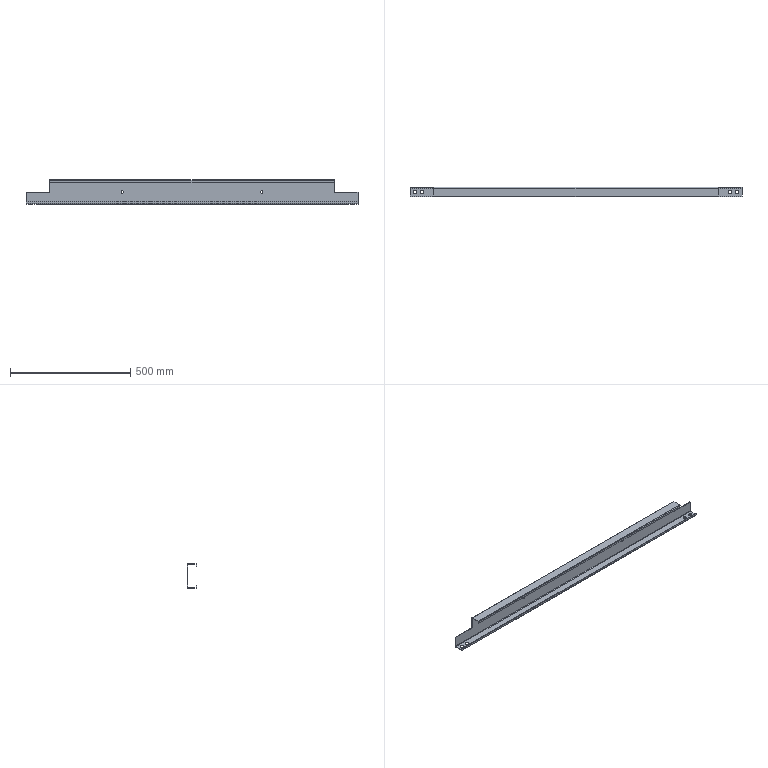Part | SolidWorks | features EdgeFlange 2, ICE 2, FlatPattern 1, SMBaseFlange 1, SheetMetal 1 | 1 solid | 54 faces | box 1380 x 40 x 100 mm | volume 478771 mm3 | plane 34 | cylinder 20 | commonest cylinder face diameters 15 x8 10 x4 2 x2 4 x2 6 x2 8 x2
STEP:
#1=CARTESIAN_POINT('',(-1204.379,-27.5,-98.));
#2=VERTEX_POINT('',#1);
#3=CARTESIAN_POINT('',(-1204.379,-12.5,-98.));
#4=VERTEX_POINT('',#3);
#5=CARTESIAN_POINT('',(-1204.379,-20.,-98.));
#6=DIRECTION('',(0.,0.,-1.));
#7=DIRECTION('',(0.,1.,0.));
#8=AXIS2_PLACEMENT_3D('',#5,#6,#7);
#9=CIRCLE('',#8,7.5);
#10=EDGE_CURVE('',#2,#4,#9,.T.);
#11=ORIENTED_EDGE('',*,*,#10,.F.);
#12=CARTESIAN_POINT('',(-1204.379,-27.5,-100.));
#13=VERTEX_POINT('',#12);
#14=CARTESIAN_POINT('',(-1204.379,-27.5,-90.));
#15=DIRECTION('',(0.,0.,-1.));
#16=VECTOR('',#15,1000.);
#17=LINE('',#14,#16);
#18=EDGE_CURVE('',#2,#13,#17,.T.);
#19=ORIENTED_EDGE('',*,*,#18,.T.);
#20=CARTESIAN_POINT('',(-1204.379,-12.5,-100.));
#21=VERTEX_POINT('',#20);
#22=CARTESIAN_POINT('',(-1204.379,-20.,-100.));
#23=DIRECTION('',(0.,0.,-1.));
#24=DIRECTION('',(0.,1.,0.));
#25=AXIS2_PLACEMENT_3D('',#22,#23,#24);
#26=CIRCLE('',#25,7.5);
#27=EDGE_CURVE('',#13,#21,#26,.T.);
#28=ORIENTED_EDGE('',*,*,#27,.T.);
#29=CARTESIAN_POINT('',(-1204.379,-12.5,-90.));
#30=DIRECTION('',(0.,0.,-1.));
#31=VECTOR('',#30,1000.);
#32=LINE('',#29,#31);
#33=EDGE_CURVE('',#4,#21,#32,.T.);
#34=ORIENTED_EDGE('',*,*,#33,.F.);
#35=EDGE_LOOP('',(#11,#19,#28,#34));
#36=FACE_OUTER_BOUND('',#35,.T.);
#37=CARTESIAN_POINT('',(-1204.379,-20.,-90.));
#38=DIRECTION('',(0.,0.,-1.));
#39=DIRECTION('',(0.,1.,0.));
#40=AXIS2_PLACEMENT_3D('',#37,#38,#39);
#41=CYLINDRICAL_SURFACE('',#40,7.5);
#42=ADVANCED_FACE('',(#36),#41,.F.);
#43=CARTESIAN_POINT('',(-1234.379,-27.5,-98.));
#44=VERTEX_POINT('',#43);
#45=CARTESIAN_POINT('',(-1234.379,-12.5,-98.));
#46=VERTEX_POINT('',#45);
#47=CARTESIAN_POINT('',(-1234.379,-20.,-98.));
#48=DIRECTION('',(0.,0.,-1.));
#49=DIRECTION('',(0.,1.,0.));
#50=AXIS2_PLACEMENT_3D('',#47,#48,#49);
#51=CIRCLE('',#50,7.5);
#52=EDGE_CURVE('',#44,#46,#51,.T.);
#53=ORIENTED_EDGE('',*,*,#52,.F.);
#54=CARTESIAN_POINT('',(-1234.379,-27.5,-100.));
#55=VERTEX_POINT('',#54);
#56=CARTESIAN_POINT('',(-1234.379,-27.5,-90.));
#57=DIRECTION('',(0.,0.,-1.));
#58=VECTOR('',#57,1000.);
#59=LINE('',#56,#58);
#60=EDGE_CURVE('',#44,#55,#59,.T.);
#61=ORIENTED_EDGE('',*,*,#60,.T.);
#62=CARTESIAN_POINT('',(-1234.379,-12.5,-100.));
#63=VERTEX_POINT('',#62);
#64=CARTESIAN_POINT('',(-1234.379,-20.,-100.));
#65=DIRECTION('',(0.,0.,-1.));
#66=DIRECTION('',(0.,1.,0.));
#67=AXIS2_PLACEMENT_3D('',#64,#65,#66);
#68=CIRCLE('',#67,7.5);
#69=EDGE_CURVE('',#55,#63,#68,.T.);
#70=ORIENTED_EDGE('',*,*,#69,.T.);
#71=CARTESIAN_POINT('',(-1234.379,-12.5,-90.));
#72=DIRECTION('',(0.,0.,-1.));
#73=VECTOR('',#72,1000.);
#74=LINE('',#71,#73);
#75=EDGE_CURVE('',#46,#63,#74,.T.);
#76=ORIENTED_EDGE('',*,*,#75,.F.);
#77=EDGE_LOOP('',(#53,#61,#70,#76));
#78=FACE_OUTER_BOUND('',#77,.T.);
#79=CARTESIAN_POINT('',(-1234.379,-20.,-90.));
#80=DIRECTION('',(0.,0.,-1.));
#81=DIRECTION('',(0.,1.,0.));
#82=AXIS2_PLACEMENT_3D('',#79,#80,#81);
#83=CYLINDRICAL_SURFACE('',#82,7.5);
#84=ADVANCED_FACE('',(#78),#83,.F.);
#85=CARTESIAN_POINT('',(75.621,-27.5,-98.));
#86=VERTEX_POINT('',#85);
#87=CARTESIAN_POINT('',(75.621,-12.5,-98.));
#88=VERTEX_POINT('',#87);
#89=CARTESIAN_POINT('',(75.621,-20.,-98.));
#90=DIRECTION('',(0.,0.,-1.));
#91=DIRECTION('',(0.,1.,0.));
#92=AXIS2_PLACEMENT_3D('',#89,#90,#91);
#93=CIRCLE('',#92,7.5);
#94=EDGE_CURVE('',#86,#88,#93,.T.);
#95=ORIENTED_EDGE('',*,*,#94,.F.);
#96=CARTESIAN_POINT('',(75.621,-27.5,-100.));
#97=VERTEX_POINT('',#96);
#98=CARTESIAN_POINT('',(75.621,-27.5,-90.));
#99=DIRECTION('',(0.,0.,-1.));
#100=VECTOR('',#99,1000.);
#101=LINE('',#98,#100);
#102=EDGE_CURVE('',#86,#97,#101,.T.);
#103=ORIENTED_EDGE('',*,*,#102,.T.);
#104=CARTESIAN_POINT('',(75.621,-12.5,-100.));
#105=VERTEX_POINT('',#104);
#106=CARTESIAN_POINT('',(75.621,-20.,-100.));
#107=DIRECTION('',(0.,0.,-1.));
#108=DIRECTION('',(0.,1.,0.));
#109=AXIS2_PLACEMENT_3D('',#106,#107,#108);
#110=CIRCLE('',#109,7.5);
#111=EDGE_CURVE('',#97,#105,#110,.T.);
#112=ORIENTED_EDGE('',*,*,#111,.T.);
#113=CARTESIAN_POINT('',(75.621,-12.5,-90.));
#114=DIRECTION('',(0.,0.,-1.));
#115=VECTOR('',#114,1000.);
#116=LINE('',#113,#115);
#117=EDGE_CURVE('',#88,#105,#116,.T.);
#118=ORIENTED_EDGE('',*,*,#117,.F.);
#119=EDGE_LOOP('',(#95,#103,#112,#118));
#120=FACE_OUTER_BOUND('',#119,.T.);
#121=CARTESIAN_POINT('',(75.621,-20.,-90.));
#122=DIRECTION('',(0.,0.,-1.));
#123=DIRECTION('',(0.,1.,0.));
#124=AXIS2_PLACEMENT_3D('',#121,#122,#123);
#125=CYLINDRICAL_SURFACE('',#124,7.5);
#126=ADVANCED_FACE('',(#120),#125,.F.);
#127=CARTESIAN_POINT('',(105.621,-27.5,-98.));
#128=VERTEX_POINT('',#127);
#129=CARTESIAN_POINT('',(105.621,-12.5,-98.));
#130=VERTEX_POINT('',#129);
#131=CARTESIAN_POINT('',(105.621,-20.,-98.));
#132=DIRECTION('',(0.,0.,-1.));
#133=DIRECTION('',(0.,1.,0.));
#134=AXIS2_PLACEMENT_3D('',#131,#132,#133);
#135=CIRCLE('',#134,7.5);
#136=EDGE_CURVE('',#128,#130,#135,.T.);
#137=ORIENTED_EDGE('',*,*,#136,.F.);
#138=CARTESIAN_POINT('',(105.621,-27.5,-100.));
#139=VERTEX_POINT('',#138);
#140=CARTESIAN_POINT('',(105.621,-27.5,-90.));
#141=DIRECTION('',(0.,0.,-1.));
#142=VECTOR('',#141,1000.);
#143=LINE('',#140,#142);
#144=EDGE_CURVE('',#128,#139,#143,.T.);
#145=ORIENTED_EDGE('',*,*,#144,.T.);
#146=CARTESIAN_POINT('',(105.621,-12.5,-100.));
#147=VERTEX_POINT('',#146);
#148=CARTESIAN_POINT('',(105.621,-20.,-100.));
#149=DIRECTION('',(0.,0.,-1.));
#150=DIRECTION('',(0.,1.,0.));
#151=AXIS2_PLACEMENT_3D('',#148,#149,#150);
#152=CIRCLE('',#151,7.5);
#153=EDGE_CURVE('',#139,#147,#152,.T.);
#154=ORIENTED_EDGE('',*,*,#153,.T.);
#155=CARTESIAN_POINT('',(105.621,-12.5,-90.));
#156=DIRECTION('',(0.,0.,-1.));
#157=VECTOR('',#156,1000.);
#158=LINE('',#155,#157);
#159=EDGE_CURVE('',#130,#147,#158,.T.);
#160=ORIENTED_EDGE('',*,*,#159,.F.);
#161=EDGE_LOOP('',(#137,#145,#154,#160));
#162=FACE_OUTER_BOUND('',#161,.T.);
#163=CARTESIAN_POINT('',(105.621,-20.,-90.));
#164=DIRECTION('',(0.,0.,-1.));
#165=DIRECTION('',(0.,1.,0.));
#166=AXIS2_PLACEMENT_3D('',#163,#164,#165);
#167=CYLINDRICAL_SURFACE('',#166,7.5);
#168=ADVANCED_FACE('',(#162),#167,.F.);
#169=CARTESIAN_POINT('',(-854.379,-2.,-55.));
#170=VERTEX_POINT('',#169);
#171=CARTESIAN_POINT('',(-854.379,-2.,-45.));
#172=VERTEX_POINT('',#171);
#173=CARTESIAN_POINT('',(-854.379,-2.,-50.));
#174=DIRECTION('',(0.,1.,0.));
#175=DIRECTION('',(0.,0.,1.));
#176=AXIS2_PLACEMENT_3D('',#173,#174,#175);
#177=CIRCLE('',#176,5.);
#178=EDGE_CURVE('',#170,#172,#177,.T.);
#179=ORIENTED_EDGE('',*,*,#178,.F.);
#180=CARTESIAN_POINT('',(-854.379,0.,-55.));
#181=VERTEX_POINT('',#180);
#182=CARTESIAN_POINT('',(-854.379,-2.,-55.));
#183=DIRECTION('',(0.,1.,0.));
#184=VECTOR('',#183,1000.);
#185=LINE('',#182,#184);
#186=EDGE_CURVE('',#170,#181,#185,.T.);
#187=ORIENTED_EDGE('',*,*,#186,.T.);
#188=CARTESIAN_POINT('',(-854.379,0.,-45.));
#189=VERTEX_POINT('',#188);
#190=CARTESIAN_POINT('',(-854.379,0.,-50.));
#191=DIRECTION('',(0.,1.,0.));
#192=DIRECTION('',(0.,0.,1.));
#193=AXIS2_PLACEMENT_3D('',#190,#191,#192);
#194=CIRCLE('',#193,5.);
#195=EDGE_CURVE('',#181,#189,#194,.T.);
#196=ORIENTED_EDGE('',*,*,#195,.T.);
#197=CARTESIAN_POINT('',(-854.379,-2.,-45.));
#198=DIRECTION('',(0.,1.,0.));
#199=VECTOR('',#198,1000.);
#200=LINE('',#197,#199);
#201=EDGE_CURVE('',#172,#189,#200,.T.);
#202=ORIENTED_EDGE('',*,*,#201,.F.);
#203=EDGE_LOOP('',(#179,#187,#196,#202));
#204=FACE_OUTER_BOUND('',#203,.T.);
#205=CARTESIAN_POINT('',(-854.379,-2.,-50.));
#206=DIRECTION('',(0.,1.,0.));
#207=DIRECTION('',(0.,0.,1.));
#208=AXIS2_PLACEMENT_3D('',#205,#206,#207);
#209=CYLINDRICAL_SURFACE('',#208,5.);
#210=ADVANCED_FACE('',(#204),#209,.F.);
#211=CARTESIAN_POINT('',(-274.379,-2.,-55.));
#212=VERTEX_POINT('',#211);
#213=CARTESIAN_POINT('',(-274.379,-2.,-45.));
#214=VERTEX_POINT('',#213);
#215=CARTESIAN_POINT('',(-274.379,-2.,-50.));
#216=DIRECTION('',(0.,1.,0.));
#217=DIRECTION('',(0.,0.,1.));
#218=AXIS2_PLACEMENT_3D('',#215,#216,#217);
#219=CIRCLE('',#218,5.);
#220=EDGE_CURVE('',#212,#214,#219,.T.);
#221=ORIENTED_EDGE('',*,*,#220,.F.);
#222=CARTESIAN_POINT('',(-274.379,0.,-55.));
#223=VERTEX_POINT('',#222);
#224=CARTESIAN_POINT('',(-274.379,-2.,-55.));
#225=DIRECTION('',(0.,1.,0.));
#226=VECTOR('',#225,1000.);
#227=LINE('',#224,#226);
#228=EDGE_CURVE('',#212,#223,#227,.T.);
#229=ORIENTED_EDGE('',*,*,#228,.T.);
#230=CARTESIAN_POINT('',(-274.379,0.,-45.));
#231=VERTEX_POINT('',#230);
#232=CARTESIAN_POINT('',(-274.379,0.,-50.));
#233=DIRECTION('',(0.,1.,0.));
#234=DIRECTION('',(0.,0.,1.));
#235=AXIS2_PLACEMENT_3D('',#232,#233,#234);
#236=CIRCLE('',#235,5.);
#237=EDGE_CURVE('',#223,#231,#236,.T.);
#238=ORIENTED_EDGE('',*,*,#237,.T.);
#239=CARTESIAN_POINT('',(-274.379,-2.,-45.));
#240=DIRECTION('',(0.,1.,0.));
#241=VECTOR('',#240,1000.);
#242=LINE('',#239,#241);
#243=EDGE_CURVE('',#214,#231,#242,.T.);
#244=ORIENTED_EDGE('',*,*,#243,.F.);
#245=EDGE_LOOP('',(#221,#229,#238,#244));
#246=FACE_OUTER_BOUND('',#245,.T.);
#247=CARTESIAN_POINT('',(-274.379,-2.,-50.));
#248=DIRECTION('',(0.,1.,0.));
#249=DIRECTION('',(0.,0.,1.));
#250=AXIS2_PLACEMENT_3D('',#247,#248,#249);
#251=CYLINDRICAL_SURFACE('',#250,5.);
#252=ADVANCED_FACE('',(#246),#251,.F.);
#253=CARTESIAN_POINT('',(-1156.379,-40.,-3.));
#254=VERTEX_POINT('',#253);
#255=CARTESIAN_POINT('',(-1156.379,-40.,-10.));
#256=VERTEX_POINT('',#255);
#257=CARTESIAN_POINT('',(-1156.379,-40.,0.));
#258=DIRECTION('',(0.,0.,-1.));
#259=VECTOR('',#258,1000.);
#260=LINE('',#257,#259);
#261=EDGE_CURVE('',#254,#256,#260,.T.);
#262=ORIENTED_EDGE('',*,*,#261,.F.);
#263=CARTESIAN_POINT('',(-1156.379,-38.,-3.));
#264=VERTEX_POINT('',#263);
#265=CARTESIAN_POINT('',(-1156.379,-40.,-3.));
#266=DIRECTION('',(0.,1.,0.));
#267=VECTOR('',#266,1000.);
#268=LINE('',#265,#267);
#269=EDGE_CURVE('',#254,#264,#268,.T.);
#270=ORIENTED_EDGE('',*,*,#269,.T.);
#271=CARTESIAN_POINT('',(-1156.379,-38.,-10.));
#272=VERTEX_POINT('',#271);
#273=CARTESIAN_POINT('',(-1156.379,-38.,0.));
#274=DIRECTION('',(0.,0.,-1.));
#275=VECTOR('',#274,1000.);
#276=LINE('',#273,#275);
#277=EDGE_CURVE('',#264,#272,#276,.T.);
#278=ORIENTED_EDGE('',*,*,#277,.T.);
#279=CARTESIAN_POINT('',(-1156.379,-40.,-10.));
#280=DIRECTION('',(0.,1.,0.));
#281=VECTOR('',#280,1000.);
#282=LINE('',#279,#281);
#283=EDGE_CURVE('',#256,#272,#282,.T.);
#284=ORIENTED_EDGE('',*,*,#283,.F.);
#285=EDGE_LOOP('',(#262,#270,#278,#284));
#286=FACE_OUTER_BOUND('',#285,.T.);
#287=CARTESIAN_POINT('',(-1156.379,24.338,-52.));
#288=DIRECTION('',(1.,0.,0.));
#289=DIRECTION('',(0.,0.,-1.));
#290=AXIS2_PLACEMENT_3D('',#287,#288,#289);
#291=PLANE('',#290);
#292=ADVANCED_FACE('',(#286),#291,.F.);
#293=CARTESIAN_POINT('',(-1156.379,-37.,-2.));
#294=VERTEX_POINT('',#293);
#295=CARTESIAN_POINT('',(-1156.379,-4.,-2.));
#296=VERTEX_POINT('',#295);
#297=CARTESIAN_POINT('',(-1156.379,0.,-2.));
#298=DIRECTION('',(0.,1.,0.));
#299=VECTOR('',#298,1000.);
#300=LINE('',#297,#299);
#301=EDGE_CURVE('',#294,#296,#300,.T.);
#302=ORIENTED_EDGE('',*,*,#301,.F.);
#303=CARTESIAN_POINT('',(-1156.379,-37.,0.));
#304=VERTEX_POINT('',#303);
#305=CARTESIAN_POINT('',(-1156.379,-37.,-2.));
#306=DIRECTION('',(0.,0.,1.));
#307=VECTOR('',#306,1000.);
#308=LINE('',#305,#307);
#309=EDGE_CURVE('',#294,#304,#308,.T.);
#310=ORIENTED_EDGE('',*,*,#309,.T.);
#311=CARTESIAN_POINT('',(-1156.379,-4.,0.));
#312=VERTEX_POINT('',#311);
#313=CARTESIAN_POINT('',(-1156.379,24.338,0.));
#314=DIRECTION('',(0.,1.,0.));
#315=VECTOR('',#314,1000.);
#316=LINE('',#313,#315);
#317=EDGE_CURVE('',#304,#312,#316,.T.);
#318=ORIENTED_EDGE('',*,*,#317,.T.);
#319=CARTESIAN_POINT('',(-1156.379,-4.,0.));
#320=DIRECTION('',(0.,0.,-1.));
#321=VECTOR('',#320,1000.);
#322=LINE('',#319,#321);
#323=EDGE_CURVE('',#312,#296,#322,.T.);
#324=ORIENTED_EDGE('',*,*,#323,.T.);
#325=EDGE_LOOP('',(#302,#310,#318,#324));
#326=FACE_OUTER_BOUND('',#325,.T.);
#327=CARTESIAN_POINT('',(-1156.379,24.338,-52.));
#328=DIRECTION('',(1.,0.,0.));
#329=DIRECTION('',(0.,0.,-1.));
#330=AXIS2_PLACEMENT_3D('',#327,#328,#329);
#331=PLANE('',#330);
#332=ADVANCED_FACE('',(#326),#331,.F.);
#333=ORIENTED_EDGE('',*,*,#269,.F.);
#334=CARTESIAN_POINT('',(-1156.379,-37.,-3.));
#335=DIRECTION('',(-1.,0.,0.));
#336=DIRECTION('',(0.,0.,-1.));
#337=AXIS2_PLACEMENT_3D('',#334,#335,#336);
#338=CIRCLE('',#337,3.);
#339=EDGE_CURVE('',#254,#304,#338,.T.);
#340=ORIENTED_EDGE('',*,*,#339,.T.);
#341=ORIENTED_EDGE('',*,*,#309,.F.);
#342=CARTESIAN_POINT('',(-1156.379,-37.,-3.));
#343=DIRECTION('',(-1.,0.,0.));
#344=DIRECTION('',(0.,0.,-1.));
#345=AXIS2_PLACEMENT_3D('',#342,#343,#344);
#346=CIRCLE('',#345,1.);
#347=EDGE_CURVE('',#264,#294,#346,.T.);
#348=ORIENTED_EDGE('',*,*,#347,.F.);
#349=EDGE_LOOP('',(#333,#340,#341,#348));
#350=FACE_OUTER_BOUND('',#349,.T.);
#351=CARTESIAN_POINT('',(-1156.379,24.338,-52.));
#352=DIRECTION('',(1.,0.,0.));
#353=DIRECTION('',(0.,0.,-1.));
#354=AXIS2_PLACEMENT_3D('',#351,#352,#353);
#355=PLANE('',#354);
#356=ADVANCED_FACE('',(#350),#355,.F.);
#357=CARTESIAN_POINT('',(-1156.379,-2.,-4.));
#358=VERTEX_POINT('',#357);
#359=CARTESIAN_POINT('',(-1156.379,-2.,-52.));
#360=VERTEX_POINT('',#359);
#361=CARTESIAN_POINT('',(-1156.379,-2.,0.));
#362=DIRECTION('',(0.,0.,-1.));
#363=VECTOR('',#362,1000.);
#364=LINE('',#361,#363);
#365=EDGE_CURVE('',#358,#360,#364,.T.);
#366=ORIENTED_EDGE('',*,*,#365,.F.);
#367=CARTESIAN_POINT('',(-1156.379,0.,-4.));
#368=VERTEX_POINT('',#367);
#369=CARTESIAN_POINT('',(-1156.379,-2.,-4.));
#370=DIRECTION('',(0.,1.,0.));
#371=VECTOR('',#370,1000.);
#372=LINE('',#369,#371);
#373=EDGE_CURVE('',#358,#368,#372,.T.);
#374=ORIENTED_EDGE('',*,*,#373,.T.);
#375=CARTESIAN_POINT('',(-1156.379,0.,-52.));
#376=VERTEX_POINT('',#375);
#377=CARTESIAN_POINT('',(-1156.379,0.,0.));
#378=DIRECTION('',(0.,0.,-1.));
#379=VECTOR('',#378,1000.);
#380=LINE('',#377,#379);
#381=EDGE_CURVE('',#368,#376,#380,.T.);
#382=ORIENTED_EDGE('',*,*,#381,.T.);
#383=CARTESIAN_POINT('',(-1156.379,24.338,-52.));
#384=DIRECTION('',(0.,1.,0.));
#385=VECTOR('',#384,1000.);
#386=LINE('',#383,#385);
#387=EDGE_CURVE('',#360,#376,#386,.T.);
#388=ORIENTED_EDGE('',*,*,#387,.F.);
#389=EDGE_LOOP('',(#366,#374,#382,#388));
#390=FACE_OUTER_BOUND('',#389,.T.);
#391=CARTESIAN_POINT('',(-1156.379,24.338,-52.));
#392=DIRECTION('',(1.,0.,0.));
#393=DIRECTION('',(0.,0.,-1.));
#394=AXIS2_PLACEMENT_3D('',#391,#392,#393);
#395=PLANE('',#394);
#396=ADVANCED_FACE('',(#390),#395,.F.);
#397=CARTESIAN_POINT('',(27.621,-38.,-10.));
#398=VERTEX_POINT('',#397);
#399=CARTESIAN_POINT('',(27.621,-38.,-3.));
#400=VERTEX_POINT('',#399);
#401=CARTESIAN_POINT('',(27.621,-38.,0.));
#402=DIRECTION('',(0.,0.,1.));
#403=VECTOR('',#402,1000.);
#404=LINE('',#401,#403);
#405=EDGE_CURVE('',#398,#400,#404,.T.);
#406=ORIENTED_EDGE('',*,*,#405,.T.);
#407=CARTESIAN_POINT('',(27.621,-40.,-3.));
#408=VERTEX_POINT('',#407);
#409=CARTESIAN_POINT('',(27.621,-38.,-3.));
#410=DIRECTION('',(0.,-1.,0.));
#411=VECTOR('',#410,1000.);
#412=LINE('',#409,#411);
#413=EDGE_CURVE('',#400,#408,#412,.T.);
#414=ORIENTED_EDGE('',*,*,#413,.T.);
#415=CARTESIAN_POINT('',(27.621,-40.,-10.));
#416=VERTEX_POINT('',#415);
#417=CARTESIAN_POINT('',(27.621,-40.,0.));
#418=DIRECTION('',(0.,0.,1.));
#419=VECTOR('',#418,1000.);
#420=LINE('',#417,#419);
#421=EDGE_CURVE('',#416,#408,#420,.T.);
#422=ORIENTED_EDGE('',*,*,#421,.F.);
#423=CARTESIAN_POINT('',(27.621,-40.,-10.));
#424=DIRECTION('',(0.,-1.,0.));
#425=VECTOR('',#424,1000.);
#426=LINE('',#423,#425);
#427=EDGE_CURVE('',#398,#416,#426,.T.);
#428=ORIENTED_EDGE('',*,*,#427,.F.);
#429=EDGE_LOOP('',(#406,#414,#422,#428));
#430=FACE_OUTER_BOUND('',#429,.T.);
#431=CARTESIAN_POINT('',(27.621,20.923,-52.));
#432=DIRECTION('',(-1.,0.,0.));
#433=DIRECTION('',(0.,-1.,0.));
#434=AXIS2_PLACEMENT_3D('',#431,#432,#433);
#435=PLANE('',#434);
#436=ADVANCED_FACE('',(#430),#435,.F.);
#437=CARTESIAN_POINT('',(27.621,-4.,0.));
#438=VERTEX_POINT('',#437);
#439=CARTESIAN_POINT('',(27.621,-37.,0.));
#440=VERTEX_POINT('',#439);
#441=CARTESIAN_POINT('',(27.621,20.923,0.));
#442=DIRECTION('',(0.,-1.,0.));
#443=VECTOR('',#442,1000.);
#444=LINE('',#441,#443);
#445=EDGE_CURVE('',#438,#440,#444,.T.);
#446=ORIENTED_EDGE('',*,*,#445,.T.);
#447=CARTESIAN_POINT('',(27.621,-37.,-2.));
#448=VERTEX_POINT('',#447);
#449=CARTESIAN_POINT('',(27.621,-37.,0.));
#450=DIRECTION('',(0.,0.,-1.));
#451=VECTOR('',#450,1000.);
#452=LINE('',#449,#451);
#453=EDGE_CURVE('',#440,#448,#452,.T.);
#454=ORIENTED_EDGE('',*,*,#453,.T.);
#455=CARTESIAN_POINT('',(27.621,-4.,-2.));
#456=VERTEX_POINT('',#455);
#457=CARTESIAN_POINT('',(27.621,0.,-2.));
#458=DIRECTION('',(0.,-1.,0.));
#459=VECTOR('',#458,1000.);
#460=LINE('',#457,#459);
#461=EDGE_CURVE('',#456,#448,#460,.T.);
#462=ORIENTED_EDGE('',*,*,#461,.F.);
#463=CARTESIAN_POINT('',(27.621,-4.,-2.));
#464=DIRECTION('',(0.,0.,1.));
#465=VECTOR('',#464,1000.);
#466=LINE('',#463,#465);
#467=EDGE_CURVE('',#456,#438,#466,.T.);
#468=ORIENTED_EDGE('',*,*,#467,.T.);
#469=EDGE_LOOP('',(#446,#454,#462,#468));
#470=FACE_OUTER_BOUND('',#469,.T.);
#471=CARTESIAN_POINT('',(27.621,20.923,-52.));
#472=DIRECTION('',(-1.,0.,0.));
#473=DIRECTION('',(0.,-1.,0.));
#474=AXIS2_PLACEMENT_3D('',#471,#472,#473);
#475=PLANE('',#474);
#476=ADVANCED_FACE('',(#470),#475,.F.);
#477=ORIENTED_EDGE('',*,*,#413,.F.);
#478=CARTESIAN_POINT('',(27.621,-37.,-3.));
#479=DIRECTION('',(1.,0.,0.));
#480=DIRECTION('',(0.,-1.,0.));
#481=AXIS2_PLACEMENT_3D('',#478,#479,#480);
#482=CIRCLE('',#481,1.);
#483=EDGE_CURVE('',#448,#400,#482,.T.);
#484=ORIENTED_EDGE('',*,*,#483,.F.);
#485=ORIENTED_EDGE('',*,*,#453,.F.);
#486=CARTESIAN_POINT('',(27.621,-37.,-3.));
#487=DIRECTION('',(1.,0.,0.));
#488=DIRECTION('',(0.,-1.,0.));
#489=AXIS2_PLACEMENT_3D('',#486,#487,#488);
#490=CIRCLE('',#489,3.);
#491=EDGE_CURVE('',#440,#408,#490,.T.);
#492=ORIENTED_EDGE('',*,*,#491,.T.);
#493=EDGE_LOOP('',(#477,#484,#485,#492));
#494=FACE_OUTER_BOUND('',#493,.T.);
#495=CARTESIAN_POINT('',(27.621,20.923,-52.));
#496=DIRECTION('',(-1.,0.,0.));
#497=DIRECTION('',(0.,-1.,0.));
#498=AXIS2_PLACEMENT_3D('',#495,#496,#497);
#499=PLANE('',#498);
#500=ADVANCED_FACE('',(#494),#499,.F.);
#501=CARTESIAN_POINT('',(27.621,0.,-52.));
#502=VERTEX_POINT('',#501);
#503=CARTESIAN_POINT('',(27.621,0.,-4.));
#504=VERTEX_POINT('',#503);
#505=CARTESIAN_POINT('',(27.621,0.,0.));
#506=DIRECTION('',(0.,0.,1.));
#507=VECTOR('',#506,1000.);
#508=LINE('',#505,#507);
#509=EDGE_CURVE('',#502,#504,#508,.T.);
#510=ORIENTED_EDGE('',*,*,#509,.T.);
#511=CARTESIAN_POINT('',(27.621,-2.,-4.));
#512=VERTEX_POINT('',#511);
#513=CARTESIAN_POINT('',(27.621,0.,-4.));
#514=DIRECTION('',(0.,-1.,0.));
#515=VECTOR('',#514,1000.);
#516=LINE('',#513,#515);
#517=EDGE_CURVE('',#504,#512,#516,.T.);
#518=ORIENTED_EDGE('',*,*,#517,.T.);
#519=CARTESIAN_POINT('',(27.621,-2.,-52.));
#520=VERTEX_POINT('',#519);
#521=CARTESIAN_POINT('',(27.621,-2.,0.));
#522=DIRECTION('',(0.,0.,1.));
#523=VECTOR('',#522,1000.);
#524=LINE('',#521,#523);
#525=EDGE_CURVE('',#520,#512,#524,.T.);
#526=ORIENTED_EDGE('',*,*,#525,.F.);
#527=CARTESIAN_POINT('',(27.621,20.923,-52.));
#528=DIRECTION('',(0.,-1.,0.));
#529=VECTOR('',#528,1000.);
#530=LINE('',#527,#529);
#531=EDGE_CURVE('',#502,#520,#530,.T.);
#532=ORIENTED_EDGE('',*,*,#531,.F.);
#533=EDGE_LOOP('',(#510,#518,#526,#532));
#534=FACE_OUTER_BOUND('',#533,.T.);
#535=CARTESIAN_POINT('',(27.621,20.923,-52.));
#536=DIRECTION('',(-1.,0.,0.));
#537=DIRECTION('',(0.,-1.,0.));
#538=AXIS2_PLACEMENT_3D('',#535,#536,#537);
#539=PLANE('',#538);
#540=ADVANCED_FACE('',(#534),#539,.F.);
#541=CARTESIAN_POINT('',(125.621,0.,-52.));
#542=VERTEX_POINT('',#541);
#543=CARTESIAN_POINT('',(125.621,0.,-96.));
#544=VERTEX_POINT('',#543);
#545=CARTESIAN_POINT('',(125.621,0.,-100.));
#546=DIRECTION('',(0.,0.,-1.));
#547=VECTOR('',#546,1000.);
#548=LINE('',#545,#547);
#549=EDGE_CURVE('',#542,#544,#548,.T.);
#550=ORIENTED_EDGE('',*,*,#549,.F.);
#551=CARTESIAN_POINT('',(125.621,-2.,-52.));
#552=VERTEX_POINT('',#551);
#553=CARTESIAN_POINT('',(125.621,-84.072,-52.));
#554=DIRECTION('',(0.,1.,0.));
#555=VECTOR('',#554,1000.);
#556=LINE('',#553,#555);
#557=EDGE_CURVE('',#552,#542,#556,.T.);
#558=ORIENTED_EDGE('',*,*,#557,.F.);
#559=CARTESIAN_POINT('',(125.621,-2.,-96.));
#560=VERTEX_POINT('',#559);
#561=CARTESIAN_POINT('',(125.621,-2.,-100.));
#562=DIRECTION('',(0.,0.,-1.));
#563=VECTOR('',#562,1000.);
#564=LINE('',#561,#563);
#565=EDGE_CURVE('',#552,#560,#564,.T.);
#566=ORIENTED_EDGE('',*,*,#565,.T.);
#567=CARTESIAN_POINT('',(125.621,-2.,-96.));
#568=DIRECTION('',(0.,1.,0.));
#569=VECTOR('',#568,1000.);
#570=LINE('',#567,#569);
#571=EDGE_CURVE('',#560,#544,#570,.T.);
#572=ORIENTED_EDGE('',*,*,#571,.T.);
#573=EDGE_LOOP('',(#550,#558,#566,#572));
#574=FACE_OUTER_BOUND('',#573,.T.);
#575=CARTESIAN_POINT('',(125.621,-2.,-100.));
#576=DIRECTION('',(1.,0.,0.));
#577=DIRECTION('',(0.,0.,-1.));
#578=AXIS2_PLACEMENT_3D('',#575,#576,#577);
#579=PLANE('',#578);
#580=ADVANCED_FACE('',(#574),#579,.T.);
#581=ORIENTED_EDGE('',*,*,#317,.F.);
#582=CARTESIAN_POINT('',(-1254.379,-37.,0.));
#583=DIRECTION('',(1.,0.,0.));
#584=VECTOR('',#583,1000.);
#585=LINE('',#582,#584);
#586=EDGE_CURVE('',#304,#440,#585,.T.);
#587=ORIENTED_EDGE('',*,*,#586,.T.);
#588=ORIENTED_EDGE('',*,*,#445,.F.);
#589=CARTESIAN_POINT('',(0.,-4.,0.));
#590=DIRECTION('',(-1.,0.,0.));
#591=VECTOR('',#590,1000.);
#592=LINE('',#589,#591);
#593=EDGE_CURVE('',#438,#312,#592,.T.);
#594=ORIENTED_EDGE('',*,*,#593,.T.);
#595=EDGE_LOOP('',(#581,#587,#588,#594));
#596=FACE_OUTER_BOUND('',#595,.T.);
#597=CARTESIAN_POINT('',(0.,0.,0.));
#598=DIRECTION('',(0.,0.,1.));
#599=DIRECTION('',(0.,-1.,0.));
#600=AXIS2_PLACEMENT_3D('',#597,#598,#599);
#601=PLANE('',#600);
#602=ADVANCED_FACE('',(#596),#601,.T.);
#603=CARTESIAN_POINT('',(-1254.379,-37.,-2.));
#604=DIRECTION('',(1.,0.,0.));
#605=VECTOR('',#604,1000.);
#606=LINE('',#603,#605);
#607=EDGE_CURVE('',#294,#448,#606,.T.);
#608=ORIENTED_EDGE('',*,*,#607,.F.);
#609=ORIENTED_EDGE('',*,*,#301,.T.);
#610=CARTESIAN_POINT('',(125.621,-4.,-2.));
#611=DIRECTION('',(-1.,0.,0.));
#612=VECTOR('',#611,1000.);
#613=LINE('',#610,#612);
#614=EDGE_CURVE('',#456,#296,#613,.T.);
#615=ORIENTED_EDGE('',*,*,#614,.F.);
#616=ORIENTED_EDGE('',*,*,#461,.T.);
#617=EDGE_LOOP('',(#608,#609,#615,#616));
#618=FACE_OUTER_BOUND('',#617,.T.);
#619=CARTESIAN_POINT('',(0.,0.,-2.));
#620=DIRECTION('',(0.,0.,1.));
#621=DIRECTION('',(0.,-1.,0.));
#622=AXIS2_PLACEMENT_3D('',#619,#620,#621);
#623=PLANE('',#622);
#624=ADVANCED_FACE('',(#618),#623,.F.);
#625=CARTESIAN_POINT('',(125.621,-37.,-98.));
#626=VERTEX_POINT('',#625);
#627=CARTESIAN_POINT('',(125.621,-4.,-98.));
#628=VERTEX_POINT('',#627);
#629=CARTESIAN_POINT('',(125.621,0.,-98.));
#630=DIRECTION('',(0.,1.,0.));
#631=VECTOR('',#630,1000.);
#632=LINE('',#629,#631);
#633=EDGE_CURVE('',#626,#628,#632,.T.);
#634=ORIENTED_EDGE('',*,*,#633,.F.);
#635=CARTESIAN_POINT('',(125.621,-37.,-100.));
#636=VERTEX_POINT('',#635);
#637=CARTESIAN_POINT('',(125.621,-37.,-98.));
#638=DIRECTION('',(0.,0.,-1.));
#639=VECTOR('',#638,1000.);
#640=LINE('',#637,#639);
#641=EDGE_CURVE('',#626,#636,#640,.T.);
#642=ORIENTED_EDGE('',*,*,#641,.T.);
#643=CARTESIAN_POINT('',(125.621,-4.,-100.));
#644=VERTEX_POINT('',#643);
#645=CARTESIAN_POINT('',(125.621,-2.,-100.));
#646=DIRECTION('',(0.,1.,0.));
#647=VECTOR('',#646,1000.);
#648=LINE('',#645,#647);
#649=EDGE_CURVE('',#636,#644,#648,.T.);
#650=ORIENTED_EDGE('',*,*,#649,.T.);
#651=CARTESIAN_POINT('',(125.621,-4.,-98.));
#652=DIRECTION('',(0.,0.,-1.));
#653=VECTOR('',#652,1000.);
#654=LINE('',#651,#653);
#655=EDGE_CURVE('',#628,#644,#654,.T.);
#656=ORIENTED_EDGE('',*,*,#655,.F.);
#657=EDGE_LOOP('',(#634,#642,#650,#656));
#658=FACE_OUTER_BOUND('',#657,.T.);
#659=CARTESIAN_POINT('',(125.621,-2.,-100.));
#660=DIRECTION('',(1.,0.,0.));
#661=DIRECTION('',(0.,0.,-1.));
#662=AXIS2_PLACEMENT_3D('',#659,#660,#661);
#663=PLANE('',#662);
#664=ADVANCED_FACE('',(#658),#663,.T.);
#665=CARTESIAN_POINT('',(-1204.379,-20.,-100.));
#666=DIRECTION('',(0.,0.,-1.));
#667=DIRECTION('',(0.,1.,0.));
#668=AXIS2_PLACEMENT_3D('',#665,#666,#667);
#669=CIRCLE('',#668,7.5);
#670=EDGE_CURVE('',#21,#13,#669,.T.);
#671=ORIENTED_EDGE('',*,*,#670,.F.);
#672=ORIENTED_EDGE('',*,*,#27,.F.);
#673=EDGE_LOOP('',(#671,#672));
#674=FACE_BOUND('',#673,.T.);
#675=CARTESIAN_POINT('',(-1234.379,-20.,-100.));
#676=DIRECTION('',(0.,0.,-1.));
#677=DIRECTION('',(0.,1.,0.));
#678=AXIS2_PLACEMENT_3D('',#675,#676,#677);
#679=CIRCLE('',#678,7.5);
#680=EDGE_CURVE('',#63,#55,#679,.T.);
#681=ORIENTED_EDGE('',*,*,#680,.F.);
#682=ORIENTED_EDGE('',*,*,#69,.F.);
#683=EDGE_LOOP('',(#681,#682));
#684=FACE_BOUND('',#683,.T.);
#685=CARTESIAN_POINT('',(75.621,-20.,-100.));
#686=DIRECTION('',(0.,0.,-1.));
#687=DIRECTION('',(0.,1.,0.));
#688=AXIS2_PLACEMENT_3D('',#685,#686,#687);
#689=CIRCLE('',#688,7.5);
#690=EDGE_CURVE('',#105,#97,#689,.T.);
#691=ORIENTED_EDGE('',*,*,#690,.F.);
#692=ORIENTED_EDGE('',*,*,#111,.F.);
#693=EDGE_LOOP('',(#691,#692));
#694=FACE_BOUND('',#693,.T.);
#695=CARTESIAN_POINT('',(105.621,-20.,-100.));
#696=DIRECTION('',(0.,0.,-1.));
#697=DIRECTION('',(0.,1.,0.));
#698=AXIS2_PLACEMENT_3D('',#695,#696,#697);
#699=CIRCLE('',#698,7.5);
#700=EDGE_CURVE('',#147,#139,#699,.T.);
#701=ORIENTED_EDGE('',*,*,#700,.F.);
#702=ORIENTED_EDGE('',*,*,#153,.F.);
#703=EDGE_LOOP('',(#701,#702));
#704=FACE_BOUND('',#703,.T.);
#705=ORIENTED_EDGE('',*,*,#649,.F.);
#706=CARTESIAN_POINT('',(-1254.379,-37.,-100.));
#707=VERTEX_POINT('',#706);
#708=CARTESIAN_POINT('',(125.621,-37.,-100.));
#709=DIRECTION('',(-1.,0.,0.));
#710=VECTOR('',#709,1000.);
#711=LINE('',#708,#710);
#712=EDGE_CURVE('',#636,#707,#711,.T.);
#713=ORIENTED_EDGE('',*,*,#712,.T.);
#714=CARTESIAN_POINT('',(-1254.379,-4.,-100.));
#715=VERTEX_POINT('',#714);
#716=CARTESIAN_POINT('',(-1254.379,-40.,-100.));
#717=DIRECTION('',(0.,-1.,0.));
#718=VECTOR('',#717,1000.);
#719=LINE('',#716,#718);
#720=EDGE_CURVE('',#715,#707,#719,.T.);
#721=ORIENTED_EDGE('',*,*,#720,.F.);
#722=CARTESIAN_POINT('',(0.,-4.,-100.));
#723=DIRECTION('',(1.,0.,0.));
#724=VECTOR('',#723,1000.);
#725=LINE('',#722,#724);
#726=EDGE_CURVE('',#715,#644,#725,.T.);
#727=ORIENTED_EDGE('',*,*,#726,.T.);
#728=EDGE_LOOP('',(#705,#713,#721,#727));
#729=FACE_OUTER_BOUND('',#728,.T.);
#730=CARTESIAN_POINT('',(0.,0.,-100.));
#731=DIRECTION('',(0.,0.,-1.));
#732=DIRECTION('',(0.,1.,0.));
#733=AXIS2_PLACEMENT_3D('',#730,#731,#732);
#734=PLANE('',#733);
#735=ADVANCED_FACE('',(#674,#684,#694,#704,#729),#734,.T.);
#736=CARTESIAN_POINT('',(-1204.379,-20.,-98.));
#737=DIRECTION('',(0.,0.,-1.));
#738=DIRECTION('',(0.,1.,0.));
#739=AXIS2_PLACEMENT_3D('',#736,#737,#738);
#740=CIRCLE('',#739,7.5);
#741=EDGE_CURVE('',#4,#2,#740,.T.);
#742=ORIENTED_EDGE('',*,*,#741,.T.);
#743=ORIENTED_EDGE('',*,*,#10,.T.);
#744=EDGE_LOOP('',(#742,#743));
#745=FACE_BOUND('',#744,.T.);
#746=CARTESIAN_POINT('',(-1234.379,-20.,-98.));
#747=DIRECTION('',(0.,0.,-1.));
#748=DIRECTION('',(0.,1.,0.));
#749=AXIS2_PLACEMENT_3D('',#746,#747,#748);
#750=CIRCLE('',#749,7.5);
#751=EDGE_CURVE('',#46,#44,#750,.T.);
#752=ORIENTED_EDGE('',*,*,#751,.T.);
#753=ORIENTED_EDGE('',*,*,#52,.T.);
#754=EDGE_LOOP('',(#752,#753));
#755=FACE_BOUND('',#754,.T.);
#756=CARTESIAN_POINT('',(75.621,-20.,-98.));
#757=DIRECTION('',(0.,0.,-1.));
#758=DIRECTION('',(0.,1.,0.));
#759=AXIS2_PLACEMENT_3D('',#756,#757,#758);
#760=CIRCLE('',#759,7.5);
#761=EDGE_CURVE('',#88,#86,#760,.T.);
#762=ORIENTED_EDGE('',*,*,#761,.T.);
#763=ORIENTED_EDGE('',*,*,#94,.T.);
#764=EDGE_LOOP('',(#762,#763));
#765=FACE_BOUND('',#764,.T.);
#766=CARTESIAN_POINT('',(105.621,-20.,-98.));
#767=DIRECTION('',(0.,0.,-1.));
#768=DIRECTION('',(0.,1.,0.));
#769=AXIS2_PLACEMENT_3D('',#766,#767,#768);
#770=CIRCLE('',#769,7.5);
#771=EDGE_CURVE('',#130,#128,#770,.T.);
#772=ORIENTED_EDGE('',*,*,#771,.T.);
#773=ORIENTED_EDGE('',*,*,#136,.T.);
#774=EDGE_LOOP('',(#772,#773));
#775=FACE_BOUND('',#774,.T.);
#776=CARTESIAN_POINT('',(-1254.379,-37.,-98.));
#777=VERTEX_POINT('',#776);
#778=CARTESIAN_POINT('',(125.621,-37.,-98.));
#779=DIRECTION('',(-1.,0.,0.));
#780=VECTOR('',#779,1000.);
#781=LINE('',#778,#780);
#782=EDGE_CURVE('',#626,#777,#781,.T.);
#783=ORIENTED_EDGE('',*,*,#782,.F.);
#784=ORIENTED_EDGE('',*,*,#633,.T.);
#785=CARTESIAN_POINT('',(-1254.379,-4.,-98.));
#786=VERTEX_POINT('',#785);
#787=CARTESIAN_POINT('',(-1254.379,-4.,-98.));
#788=DIRECTION('',(1.,0.,0.));
#789=VECTOR('',#788,1000.);
#790=LINE('',#787,#789);
#791=EDGE_CURVE('',#786,#628,#790,.T.);
#792=ORIENTED_EDGE('',*,*,#791,.F.);
#793=CARTESIAN_POINT('',(-1254.379,0.,-98.));
#794=DIRECTION('',(0.,-1.,0.));
#795=VECTOR('',#794,1000.);
#796=LINE('',#793,#795);
#797=EDGE_CURVE('',#786,#777,#796,.T.);
#798=ORIENTED_EDGE('',*,*,#797,.T.);
#799=EDGE_LOOP('',(#783,#784,#792,#798));
#800=FACE_OUTER_BOUND('',#799,.T.);
#801=CARTESIAN_POINT('',(0.,0.,-98.));
#802=DIRECTION('',(0.,0.,-1.));
#803=DIRECTION('',(0.,1.,0.));
#804=AXIS2_PLACEMENT_3D('',#801,#802,#803);
#805=PLANE('',#804);
#806=ADVANCED_FACE('',(#745,#755,#765,#775,#800),#805,.F.);
#807=CARTESIAN_POINT('',(-854.379,-2.,-50.));
#808=DIRECTION('',(0.,1.,0.));
#809=DIRECTION('',(0.,0.,1.));
#810=AXIS2_PLACEMENT_3D('',#807,#808,#809);
#811=CIRCLE('',#810,5.);
#812=EDGE_CURVE('',#172,#170,#811,.T.);
#813=ORIENTED_EDGE('',*,*,#812,.T.);
#814=ORIENTED_EDGE('',*,*,#178,.T.);
#815=EDGE_LOOP('',(#813,#814));
#816=FACE_BOUND('',#815,.T.);
#817=CARTESIAN_POINT('',(-274.379,-2.,-50.));
#818=DIRECTION('',(0.,1.,0.));
#819=DIRECTION('',(0.,0.,1.));
#820=AXIS2_PLACEMENT_3D('',#817,#818,#819);
#821=CIRCLE('',#820,5.);
#822=EDGE_CURVE('',#214,#212,#821,.T.);
#823=ORIENTED_EDGE('',*,*,#822,.T.);
#824=ORIENTED_EDGE('',*,*,#220,.T.);
#825=EDGE_LOOP('',(#823,#824));
#826=FACE_BOUND('',#825,.T.);
#827=CARTESIAN_POINT('',(-1254.379,-2.,-4.));
#828=DIRECTION('',(1.,0.,0.));
#829=VECTOR('',#828,1000.);
#830=LINE('',#827,#829);
#831=EDGE_CURVE('',#358,#512,#830,.T.);
#832=ORIENTED_EDGE('',*,*,#831,.F.);
#833=ORIENTED_EDGE('',*,*,#365,.T.);
#834=CARTESIAN_POINT('',(-1254.379,-2.,-52.));
#835=VERTEX_POINT('',#834);
#836=CARTESIAN_POINT('',(0.,-2.,-52.));
#837=DIRECTION('',(-1.,0.,0.));
#838=VECTOR('',#837,1000.);
#839=LINE('',#836,#838);
#840=EDGE_CURVE('',#360,#835,#839,.T.);
#841=ORIENTED_EDGE('',*,*,#840,.T.);
#842=CARTESIAN_POINT('',(-1254.379,-2.,-96.));
#843=VERTEX_POINT('',#842);
#844=CARTESIAN_POINT('',(-1254.379,-2.,-100.));
#845=DIRECTION('',(0.,0.,1.));
#846=VECTOR('',#845,1000.);
#847=LINE('',#844,#846);
#848=EDGE_CURVE('',#843,#835,#847,.T.);
#849=ORIENTED_EDGE('',*,*,#848,.F.);
#850=CARTESIAN_POINT('',(125.621,-2.,-96.));
#851=DIRECTION('',(-1.,0.,0.));
#852=VECTOR('',#851,1000.);
#853=LINE('',#850,#852);
#854=EDGE_CURVE('',#560,#843,#853,.T.);
#855=ORIENTED_EDGE('',*,*,#854,.F.);
#856=ORIENTED_EDGE('',*,*,#565,.F.);
#857=CARTESIAN_POINT('',(0.,-2.,-52.));
#858=DIRECTION('',(1.,0.,0.));
#859=VECTOR('',#858,1000.);
#860=LINE('',#857,#859);
#861=EDGE_CURVE('',#520,#552,#860,.T.);
#862=ORIENTED_EDGE('',*,*,#861,.F.);
#863=ORIENTED_EDGE('',*,*,#525,.T.);
#864=EDGE_LOOP('',(#832,#833,#841,#849,#855,#856,#862,#863));
#865=FACE_OUTER_BOUND('',#864,.T.);
#866=CARTESIAN_POINT('',(0.,-2.,0.));
#867=DIRECTION('',(0.,1.,0.));
#868=DIRECTION('',(0.,0.,1.));
#869=AXIS2_PLACEMENT_3D('',#866,#867,#868);
#870=PLANE('',#869);
#871=ADVANCED_FACE('',(#816,#826,#865),#870,.F.);
#872=ORIENTED_EDGE('',*,*,#381,.F.);
#873=CARTESIAN_POINT('',(-1254.379,0.,-4.));
#874=DIRECTION('',(1.,0.,0.));
#875=VECTOR('',#874,1000.);
#876=LINE('',#873,#875);
#877=EDGE_CURVE('',#368,#504,#876,.T.);
#878=ORIENTED_EDGE('',*,*,#877,.T.);
#879=ORIENTED_EDGE('',*,*,#509,.F.);
#880=CARTESIAN_POINT('',(0.,0.,-52.));
#881=DIRECTION('',(1.,0.,0.));
#882=VECTOR('',#881,1000.);
#883=LINE('',#880,#882);
#884=EDGE_CURVE('',#502,#542,#883,.T.);
#885=ORIENTED_EDGE('',*,*,#884,.T.);
#886=ORIENTED_EDGE('',*,*,#549,.T.);
#887=CARTESIAN_POINT('',(-1254.379,0.,-96.));
#888=VERTEX_POINT('',#887);
#889=CARTESIAN_POINT('',(125.621,0.,-96.));
#890=DIRECTION('',(-1.,0.,0.));
#891=VECTOR('',#890,1000.);
#892=LINE('',#889,#891);
#893=EDGE_CURVE('',#544,#888,#892,.T.);
#894=ORIENTED_EDGE('',*,*,#893,.T.);
#895=CARTESIAN_POINT('',(-1254.379,0.,-52.));
#896=VERTEX_POINT('',#895);
#897=CARTESIAN_POINT('',(-1254.379,0.,-100.));
#898=DIRECTION('',(0.,0.,1.));
#899=VECTOR('',#898,1000.);
#900=LINE('',#897,#899);
#901=EDGE_CURVE('',#888,#896,#900,.T.);
#902=ORIENTED_EDGE('',*,*,#901,.T.);
#903=CARTESIAN_POINT('',(0.,0.,-52.));
#904=DIRECTION('',(-1.,0.,0.));
#905=VECTOR('',#904,1000.);
#906=LINE('',#903,#905);
#907=EDGE_CURVE('',#376,#896,#906,.T.);
#908=ORIENTED_EDGE('',*,*,#907,.F.);
#909=EDGE_LOOP('',(#872,#878,#879,#885,#886,#894,#902,#908));
#910=FACE_OUTER_BOUND('',#909,.T.);
#911=CARTESIAN_POINT('',(-854.379,0.,-50.));
#912=DIRECTION('',(0.,1.,0.));
#913=DIRECTION('',(0.,0.,1.));
#914=AXIS2_PLACEMENT_3D('',#911,#912,#913);
#915=CIRCLE('',#914,5.);
#916=EDGE_CURVE('',#189,#181,#915,.T.);
#917=ORIENTED_EDGE('',*,*,#916,.F.);
#918=ORIENTED_EDGE('',*,*,#195,.F.);
#919=EDGE_LOOP('',(#917,#918));
#920=FACE_BOUND('',#919,.T.);
#921=CARTESIAN_POINT('',(-274.379,0.,-50.));
#922=DIRECTION('',(0.,1.,0.));
#923=DIRECTION('',(0.,0.,1.));
#924=AXIS2_PLACEMENT_3D('',#921,#922,#923);
#925=CIRCLE('',#924,5.);
#926=EDGE_CURVE('',#231,#223,#925,.T.);
#927=ORIENTED_EDGE('',*,*,#926,.F.);
#928=ORIENTED_EDGE('',*,*,#237,.F.);
#929=EDGE_LOOP('',(#927,#928));
#930=FACE_BOUND('',#929,.T.);
#931=CARTESIAN_POINT('',(0.,0.,0.));
#932=DIRECTION('',(0.,1.,0.));
#933=DIRECTION('',(0.,0.,1.));
#934=AXIS2_PLACEMENT_3D('',#931,#932,#933);
#935=PLANE('',#934);
#936=ADVANCED_FACE('',(#910,#920,#930),#935,.T.);
#937=CARTESIAN_POINT('',(-1254.379,-37.,-52.));
#938=DIRECTION('',(0.,-1.,0.));
#939=VECTOR('',#938,1000.);
#940=LINE('',#937,#939);
#941=EDGE_CURVE('',#896,#835,#940,.T.);
#942=ORIENTED_EDGE('',*,*,#941,.F.);
#943=ORIENTED_EDGE('',*,*,#901,.F.);
#944=CARTESIAN_POINT('',(-1254.379,-2.,-96.));
#945=DIRECTION('',(0.,1.,0.));
#946=VECTOR('',#945,1000.);
#947=LINE('',#944,#946);
#948=EDGE_CURVE('',#843,#888,#947,.T.);
#949=ORIENTED_EDGE('',*,*,#948,.F.);
#950=ORIENTED_EDGE('',*,*,#848,.T.);
#951=EDGE_LOOP('',(#942,#943,#949,#950));
#952=FACE_OUTER_BOUND('',#951,.T.);
#953=CARTESIAN_POINT('',(-1254.379,-2.,-100.));
#954=DIRECTION('',(-1.,0.,0.));
#955=DIRECTION('',(0.,0.,1.));
#956=AXIS2_PLACEMENT_3D('',#953,#954,#955);
#957=PLANE('',#956);
#958=ADVANCED_FACE('',(#952),#957,.T.);
#959=ORIENTED_EDGE('',*,*,#228,.F.);
#960=ORIENTED_EDGE('',*,*,#822,.F.);
#961=ORIENTED_EDGE('',*,*,#243,.T.);
#962=ORIENTED_EDGE('',*,*,#926,.T.);
#963=EDGE_LOOP('',(#959,#960,#961,#962));
#964=FACE_OUTER_BOUND('',#963,.T.);
#965=CARTESIAN_POINT('',(-274.379,-2.,-50.));
#966=DIRECTION('',(0.,1.,0.));
#967=DIRECTION('',(0.,0.,1.));
#968=AXIS2_PLACEMENT_3D('',#965,#966,#967);
#969=CYLINDRICAL_SURFACE('',#968,5.);
#970=ADVANCED_FACE('',(#964),#969,.F.);
#971=ORIENTED_EDGE('',*,*,#186,.F.);
#972=ORIENTED_EDGE('',*,*,#812,.F.);
#973=ORIENTED_EDGE('',*,*,#201,.T.);
#974=ORIENTED_EDGE('',*,*,#916,.T.);
#975=EDGE_LOOP('',(#971,#972,#973,#974));
#976=FACE_OUTER_BOUND('',#975,.T.);
#977=CARTESIAN_POINT('',(-854.379,-2.,-50.));
#978=DIRECTION('',(0.,1.,0.));
#979=DIRECTION('',(0.,0.,1.));
#980=AXIS2_PLACEMENT_3D('',#977,#978,#979);
#981=CYLINDRICAL_SURFACE('',#980,5.);
#982=ADVANCED_FACE('',(#976),#981,.F.);
#983=CARTESIAN_POINT('',(-1156.379,-4.,-4.));
#984=DIRECTION('',(-1.,0.,0.));
#985=DIRECTION('',(0.,0.,-1.));
#986=AXIS2_PLACEMENT_3D('',#983,#984,#985);
#987=CIRCLE('',#986,4.);
#988=EDGE_CURVE('',#312,#368,#987,.T.);
#989=ORIENTED_EDGE('',*,*,#988,.F.);
#990=ORIENTED_EDGE('',*,*,#593,.F.);
#991=CARTESIAN_POINT('',(27.621,-4.,-4.));
#992=DIRECTION('',(1.,0.,0.));
#993=DIRECTION('',(0.,-1.,0.));
#994=AXIS2_PLACEMENT_3D('',#991,#992,#993);
#995=CIRCLE('',#994,4.);
#996=EDGE_CURVE('',#504,#438,#995,.T.);
#997=ORIENTED_EDGE('',*,*,#996,.F.);
#998=ORIENTED_EDGE('',*,*,#877,.F.);
#999=EDGE_LOOP('',(#989,#990,#997,#998));
#1000=FACE_OUTER_BOUND('',#999,.T.);
#1001=CARTESIAN_POINT('',(-1254.379,-4.,-4.));
#1002=DIRECTION('',(-1.,0.,0.));
#1003=DIRECTION('',(0.,0.,1.));
#1004=AXIS2_PLACEMENT_3D('',#1001,#1002,#1003);
#1005=CYLINDRICAL_SURFACE('',#1004,4.);
#1006=ADVANCED_FACE('',(#1000),#1005,.T.);
#1007=ORIENTED_EDGE('',*,*,#614,.T.);
#1008=CARTESIAN_POINT('',(-1156.379,-4.,-4.));
#1009=DIRECTION('',(-1.,0.,0.));
#1010=DIRECTION('',(0.,0.,-1.));
#1011=AXIS2_PLACEMENT_3D('',#1008,#1009,#1010);
#1012=CIRCLE('',#1011,2.);
#1013=EDGE_CURVE('',#296,#358,#1012,.T.);
#1014=ORIENTED_EDGE('',*,*,#1013,.T.);
#1015=ORIENTED_EDGE('',*,*,#831,.T.);
#1016=CARTESIAN_POINT('',(27.621,-4.,-4.));
#1017=DIRECTION('',(1.,0.,0.));
#1018=DIRECTION('',(0.,-1.,0.));
#1019=AXIS2_PLACEMENT_3D('',#1016,#1017,#1018);
#1020=CIRCLE('',#1019,2.);
#1021=EDGE_CURVE('',#512,#456,#1020,.T.);
#1022=ORIENTED_EDGE('',*,*,#1021,.T.);
#1023=EDGE_LOOP('',(#1007,#1014,#1015,#1022));
#1024=FACE_OUTER_BOUND('',#1023,.T.);
#1025=CARTESIAN_POINT('',(-1254.379,-4.,-4.));
#1026=DIRECTION('',(-1.,0.,0.));
#1027=DIRECTION('',(0.,0.,1.));
#1028=AXIS2_PLACEMENT_3D('',#1025,#1026,#1027);
#1029=CYLINDRICAL_SURFACE('',#1028,2.);
#1030=ADVANCED_FACE('',(#1024),#1029,.F.);
#1031=CARTESIAN_POINT('',(-1254.379,-4.,-100.));
#1032=DIRECTION('',(0.,0.,-1.));
#1033=VECTOR('',#1032,1000.);
#1034=LINE('',#1031,#1033);
#1035=EDGE_CURVE('',#786,#715,#1034,.T.);
#1036=ORIENTED_EDGE('',*,*,#1035,.F.);
#1037=CARTESIAN_POINT('',(-1254.379,-4.,-96.));
#1038=DIRECTION('',(-1.,0.,0.));
#1039=DIRECTION('',(0.,0.,-1.));
#1040=AXIS2_PLACEMENT_3D('',#1037,#1038,#1039);
#1041=CIRCLE('',#1040,2.);
#1042=EDGE_CURVE('',#843,#786,#1041,.T.);
#1043=ORIENTED_EDGE('',*,*,#1042,.F.);
#1044=ORIENTED_EDGE('',*,*,#948,.T.);
#1045=CARTESIAN_POINT('',(-1254.379,-4.,-96.));
#1046=DIRECTION('',(-1.,0.,0.));
#1047=DIRECTION('',(0.,0.,-1.));
#1048=AXIS2_PLACEMENT_3D('',#1045,#1046,#1047);
#1049=CIRCLE('',#1048,4.);
#1050=EDGE_CURVE('',#888,#715,#1049,.T.);
#1051=ORIENTED_EDGE('',*,*,#1050,.T.);
#1052=EDGE_LOOP('',(#1036,#1043,#1044,#1051));
#1053=FACE_OUTER_BOUND('',#1052,.T.);
#1054=CARTESIAN_POINT('',(-1254.379,-4.,-96.));
#1055=DIRECTION('',(-1.,0.,0.));
#1056=DIRECTION('',(0.,0.,1.));
#1057=AXIS2_PLACEMENT_3D('',#1054,#1055,#1056);
#1058=PLANE('',#1057);
#1059=ADVANCED_FACE('',(#1053),#1058,.T.);
#1060=CARTESIAN_POINT('',(125.621,-4.,-96.));
#1061=DIRECTION('',(1.,0.,0.));
#1062=DIRECTION('',(0.,0.,-1.));
#1063=AXIS2_PLACEMENT_3D('',#1060,#1061,#1062);
#1064=CIRCLE('',#1063,2.);
#1065=EDGE_CURVE('',#628,#560,#1064,.T.);
#1066=ORIENTED_EDGE('',*,*,#1065,.F.);
#1067=ORIENTED_EDGE('',*,*,#655,.T.);
#1068=CARTESIAN_POINT('',(125.621,-4.,-96.));
#1069=DIRECTION('',(1.,0.,0.));
#1070=DIRECTION('',(0.,0.,-1.));
#1071=AXIS2_PLACEMENT_3D('',#1068,#1069,#1070);
#1072=CIRCLE('',#1071,4.);
#1073=EDGE_CURVE('',#644,#544,#1072,.T.);
#1074=ORIENTED_EDGE('',*,*,#1073,.T.);
#1075=ORIENTED_EDGE('',*,*,#571,.F.);
#1076=EDGE_LOOP('',(#1066,#1067,#1074,#1075));
#1077=FACE_OUTER_BOUND('',#1076,.T.);
#1078=CARTESIAN_POINT('',(125.621,-4.,-96.));
#1079=DIRECTION('',(-1.,0.,0.));
#1080=DIRECTION('',(0.,0.,1.));
#1081=AXIS2_PLACEMENT_3D('',#1078,#1079,#1080);
#1082=PLANE('',#1081);
#1083=ADVANCED_FACE('',(#1077),#1082,.F.);
#1084=ORIENTED_EDGE('',*,*,#893,.F.);
#1085=ORIENTED_EDGE('',*,*,#1073,.F.);
#1086=ORIENTED_EDGE('',*,*,#726,.F.);
#1087=ORIENTED_EDGE('',*,*,#1050,.F.);
#1088=EDGE_LOOP('',(#1084,#1085,#1086,#1087));
#1089=FACE_OUTER_BOUND('',#1088,.T.);
#1090=CARTESIAN_POINT('',(125.621,-4.,-96.));
#1091=DIRECTION('',(1.,0.,0.));
#1092=DIRECTION('',(0.,0.,-1.));
#1093=AXIS2_PLACEMENT_3D('',#1090,#1091,#1092);
#1094=CYLINDRICAL_SURFACE('',#1093,4.);
#1095=ADVANCED_FACE('',(#1089),#1094,.T.);
#1096=ORIENTED_EDGE('',*,*,#854,.T.);
#1097=ORIENTED_EDGE('',*,*,#1042,.T.);
#1098=ORIENTED_EDGE('',*,*,#791,.T.);
#1099=ORIENTED_EDGE('',*,*,#1065,.T.);
#1100=EDGE_LOOP('',(#1096,#1097,#1098,#1099));
#1101=FACE_OUTER_BOUND('',#1100,.T.);
#1102=CARTESIAN_POINT('',(125.621,-4.,-96.));
#1103=DIRECTION('',(1.,0.,0.));
#1104=DIRECTION('',(0.,0.,-1.));
#1105=AXIS2_PLACEMENT_3D('',#1102,#1103,#1104);
#1106=CYLINDRICAL_SURFACE('',#1105,2.);
#1107=ADVANCED_FACE('',(#1101),#1106,.F.);
#1108=CARTESIAN_POINT('',(-1254.379,-37.,-98.));
#1109=DIRECTION('',(0.,0.,-1.));
#1110=VECTOR('',#1109,1000.);
#1111=LINE('',#1108,#1110);
#1112=EDGE_CURVE('',#777,#707,#1111,.T.);
#1113=ORIENTED_EDGE('',*,*,#1112,.F.);
#1114=ORIENTED_EDGE('',*,*,#797,.F.);
#1115=ORIENTED_EDGE('',*,*,#1035,.T.);
#1116=ORIENTED_EDGE('',*,*,#720,.T.);
#1117=EDGE_LOOP('',(#1113,#1114,#1115,#1116));
#1118=FACE_OUTER_BOUND('',#1117,.T.);
#1119=CARTESIAN_POINT('',(-1254.379,-40.,-100.));
#1120=DIRECTION('',(-1.,0.,0.));
#1121=DIRECTION('',(0.,0.,1.));
#1122=AXIS2_PLACEMENT_3D('',#1119,#1120,#1121);
#1123=PLANE('',#1122);
#1124=ADVANCED_FACE('',(#1118),#1123,.T.);
#1125=CARTESIAN_POINT('',(-1254.379,-38.,-97.));
#1126=VERTEX_POINT('',#1125);
#1127=CARTESIAN_POINT('',(-1254.379,-40.,-97.));
#1128=VERTEX_POINT('',#1127);
#1129=CARTESIAN_POINT('',(-1254.379,-40.,-97.));
#1130=DIRECTION('',(0.,-1.,0.));
#1131=VECTOR('',#1130,1000.);
#1132=LINE('',#1129,#1131);
#1133=EDGE_CURVE('',#1126,#1128,#1132,.T.);
#1134=ORIENTED_EDGE('',*,*,#1133,.F.);
#1135=CARTESIAN_POINT('',(-1254.379,-37.,-97.));
#1136=DIRECTION('',(-1.,0.,0.));
#1137=DIRECTION('',(0.,0.,-1.));
#1138=AXIS2_PLACEMENT_3D('',#1135,#1136,#1137);
#1139=CIRCLE('',#1138,1.);
#1140=EDGE_CURVE('',#777,#1126,#1139,.T.);
#1141=ORIENTED_EDGE('',*,*,#1140,.F.);
#1142=ORIENTED_EDGE('',*,*,#1112,.T.);
#1143=CARTESIAN_POINT('',(-1254.379,-37.,-97.));
#1144=DIRECTION('',(-1.,0.,0.));
#1145=DIRECTION('',(0.,0.,-1.));
#1146=AXIS2_PLACEMENT_3D('',#1143,#1144,#1145);
#1147=CIRCLE('',#1146,3.);
#1148=EDGE_CURVE('',#707,#1128,#1147,.T.);
#1149=ORIENTED_EDGE('',*,*,#1148,.T.);
#1150=EDGE_LOOP('',(#1134,#1141,#1142,#1149));
#1151=FACE_OUTER_BOUND('',#1150,.T.);
#1152=CARTESIAN_POINT('',(-1254.379,-37.,-97.));
#1153=DIRECTION('',(-1.,0.,0.));
#1154=DIRECTION('',(0.,0.,1.));
#1155=AXIS2_PLACEMENT_3D('',#1152,#1153,#1154);
#1156=PLANE('',#1155);
#1157=ADVANCED_FACE('',(#1151),#1156,.T.);
#1158=CARTESIAN_POINT('',(125.621,-38.,-97.));
#1159=VERTEX_POINT('',#1158);
#1160=CARTESIAN_POINT('',(125.621,-37.,-97.));
#1161=DIRECTION('',(1.,0.,0.));
#1162=DIRECTION('',(0.,0.,-1.));
#1163=AXIS2_PLACEMENT_3D('',#1160,#1161,#1162);
#1164=CIRCLE('',#1163,1.);
#1165=EDGE_CURVE('',#1159,#626,#1164,.T.);
#1166=ORIENTED_EDGE('',*,*,#1165,.F.);
#1167=CARTESIAN_POINT('',(125.621,-40.,-97.));
#1168=VERTEX_POINT('',#1167);
#1169=CARTESIAN_POINT('',(125.621,-38.,-97.));
#1170=DIRECTION('',(0.,-1.,0.));
#1171=VECTOR('',#1170,1000.);
#1172=LINE('',#1169,#1171);
#1173=EDGE_CURVE('',#1159,#1168,#1172,.T.);
#1174=ORIENTED_EDGE('',*,*,#1173,.T.);
#1175=CARTESIAN_POINT('',(125.621,-37.,-97.));
#1176=DIRECTION('',(1.,0.,0.));
#1177=DIRECTION('',(0.,0.,-1.));
#1178=AXIS2_PLACEMENT_3D('',#1175,#1176,#1177);
#1179=CIRCLE('',#1178,3.);
#1180=EDGE_CURVE('',#1168,#636,#1179,.T.);
#1181=ORIENTED_EDGE('',*,*,#1180,.T.);
#1182=ORIENTED_EDGE('',*,*,#641,.F.);
#1183=EDGE_LOOP('',(#1166,#1174,#1181,#1182));
#1184=FACE_OUTER_BOUND('',#1183,.T.);
#1185=CARTESIAN_POINT('',(125.621,-37.,-97.));
#1186=DIRECTION('',(-1.,0.,0.));
#1187=DIRECTION('',(0.,0.,1.));
#1188=AXIS2_PLACEMENT_3D('',#1185,#1186,#1187);
#1189=PLANE('',#1188);
#1190=ADVANCED_FACE('',(#1184),#1189,.F.);
#1191=ORIENTED_EDGE('',*,*,#712,.F.);
#1192=ORIENTED_EDGE('',*,*,#1180,.F.);
#1193=CARTESIAN_POINT('',(-1254.379,-40.,-97.));
#1194=DIRECTION('',(-1.,0.,0.));
#1195=VECTOR('',#1194,1000.);
#1196=LINE('',#1193,#1195);
#1197=EDGE_CURVE('',#1168,#1128,#1196,.T.);
#1198=ORIENTED_EDGE('',*,*,#1197,.T.);
#1199=ORIENTED_EDGE('',*,*,#1148,.F.);
#1200=EDGE_LOOP('',(#1191,#1192,#1198,#1199));
#1201=FACE_OUTER_BOUND('',#1200,.T.);
#1202=CARTESIAN_POINT('',(125.621,-37.,-97.));
#1203=DIRECTION('',(1.,0.,0.));
#1204=DIRECTION('',(0.,-1.,0.));
#1205=AXIS2_PLACEMENT_3D('',#1202,#1203,#1204);
#1206=CYLINDRICAL_SURFACE('',#1205,3.);
#1207=ADVANCED_FACE('',(#1201),#1206,.T.);
#1208=ORIENTED_EDGE('',*,*,#782,.T.);
#1209=ORIENTED_EDGE('',*,*,#1140,.T.);
#1210=CARTESIAN_POINT('',(-1254.379,-38.,-97.));
#1211=DIRECTION('',(1.,0.,0.));
#1212=VECTOR('',#1211,1000.);
#1213=LINE('',#1210,#1212);
#1214=EDGE_CURVE('',#1126,#1159,#1213,.T.);
#1215=ORIENTED_EDGE('',*,*,#1214,.T.);
#1216=ORIENTED_EDGE('',*,*,#1165,.T.);
#1217=EDGE_LOOP('',(#1208,#1209,#1215,#1216));
#1218=FACE_OUTER_BOUND('',#1217,.T.);
#1219=CARTESIAN_POINT('',(125.621,-37.,-97.));
#1220=DIRECTION('',(1.,0.,0.));
#1221=DIRECTION('',(0.,-1.,0.));
#1222=AXIS2_PLACEMENT_3D('',#1219,#1220,#1221);
#1223=CYLINDRICAL_SURFACE('',#1222,1.);
#1224=ADVANCED_FACE('',(#1218),#1223,.F.);
#1225=ORIENTED_EDGE('',*,*,#1173,.F.);
#1226=CARTESIAN_POINT('',(125.621,-38.,-90.));
#1227=VERTEX_POINT('',#1226);
#1228=CARTESIAN_POINT('',(125.621,-38.,-90.));
#1229=DIRECTION('',(0.,0.,1.));
#1230=VECTOR('',#1229,1000.);
#1231=LINE('',#1228,#1230);
#1232=EDGE_CURVE('',#1159,#1227,#1231,.T.);
#1233=ORIENTED_EDGE('',*,*,#1232,.T.);
#1234=CARTESIAN_POINT('',(125.621,-40.,-90.));
#1235=VERTEX_POINT('',#1234);
#1236=CARTESIAN_POINT('',(125.621,-40.,-90.));
#1237=DIRECTION('',(0.,1.,0.));
#1238=VECTOR('',#1237,1000.);
#1239=LINE('',#1236,#1238);
#1240=EDGE_CURVE('',#1235,#1227,#1239,.T.);
#1241=ORIENTED_EDGE('',*,*,#1240,.F.);
#1242=CARTESIAN_POINT('',(125.621,-40.,0.));
#1243=DIRECTION('',(0.,0.,1.));
#1244=VECTOR('',#1243,1000.);
#1245=LINE('',#1242,#1244);
#1246=EDGE_CURVE('',#1168,#1235,#1245,.T.);
#1247=ORIENTED_EDGE('',*,*,#1246,.F.);
#1248=EDGE_LOOP('',(#1225,#1233,#1241,#1247));
#1249=FACE_OUTER_BOUND('',#1248,.T.);
#1250=CARTESIAN_POINT('',(125.621,-40.,-90.));
#1251=DIRECTION('',(-1.,0.,0.));
#1252=DIRECTION('',(0.,0.,1.));
#1253=AXIS2_PLACEMENT_3D('',#1250,#1251,#1252);
#1254=PLANE('',#1253);
#1255=ADVANCED_FACE('',(#1249),#1254,.F.);
#1256=ORIENTED_EDGE('',*,*,#1133,.T.);
#1257=CARTESIAN_POINT('',(-1254.379,-40.,-90.));
#1258=VERTEX_POINT('',#1257);
#1259=CARTESIAN_POINT('',(-1254.379,-40.,0.));
#1260=DIRECTION('',(0.,0.,-1.));
#1261=VECTOR('',#1260,1000.);
#1262=LINE('',#1259,#1261);
#1263=EDGE_CURVE('',#1258,#1128,#1262,.T.);
#1264=ORIENTED_EDGE('',*,*,#1263,.F.);
#1265=CARTESIAN_POINT('',(-1254.379,-38.,-90.));
#1266=VERTEX_POINT('',#1265);
#1267=CARTESIAN_POINT('',(-1254.379,-40.,-90.));
#1268=DIRECTION('',(0.,1.,0.));
#1269=VECTOR('',#1268,1000.);
#1270=LINE('',#1267,#1269);
#1271=EDGE_CURVE('',#1258,#1266,#1270,.T.);
#1272=ORIENTED_EDGE('',*,*,#1271,.T.);
#1273=CARTESIAN_POINT('',(-1254.379,-38.,-98.));
#1274=DIRECTION('',(0.,0.,-1.));
#1275=VECTOR('',#1274,1000.);
#1276=LINE('',#1273,#1275);
#1277=EDGE_CURVE('',#1266,#1126,#1276,.T.);
#1278=ORIENTED_EDGE('',*,*,#1277,.T.);
#1279=EDGE_LOOP('',(#1256,#1264,#1272,#1278));
#1280=FACE_OUTER_BOUND('',#1279,.T.);
#1281=CARTESIAN_POINT('',(-1254.379,-40.,-98.));
#1282=DIRECTION('',(1.,0.,0.));
#1283=DIRECTION('',(0.,0.,-1.));
#1284=AXIS2_PLACEMENT_3D('',#1281,#1282,#1283);
#1285=PLANE('',#1284);
#1286=ADVANCED_FACE('',(#1280),#1285,.F.);
#1287=ORIENTED_EDGE('',*,*,#1197,.F.);
#1288=ORIENTED_EDGE('',*,*,#1246,.T.);
#1289=CARTESIAN_POINT('',(0.,-40.,-90.));
#1290=DIRECTION('',(-1.,0.,0.));
#1291=VECTOR('',#1290,1000.);
#1292=LINE('',#1289,#1291);
#1293=EDGE_CURVE('',#1235,#1258,#1292,.T.);
#1294=ORIENTED_EDGE('',*,*,#1293,.T.);
#1295=ORIENTED_EDGE('',*,*,#1263,.T.);
#1296=EDGE_LOOP('',(#1287,#1288,#1294,#1295));
#1297=FACE_OUTER_BOUND('',#1296,.T.);
#1298=CARTESIAN_POINT('',(0.,-40.,0.));
#1299=DIRECTION('',(0.,1.,0.));
#1300=DIRECTION('',(0.,0.,1.));
#1301=AXIS2_PLACEMENT_3D('',#1298,#1299,#1300);
#1302=PLANE('',#1301);
#1303=ADVANCED_FACE('',(#1297),#1302,.F.);
#1304=ORIENTED_EDGE('',*,*,#1232,.F.);
#1305=ORIENTED_EDGE('',*,*,#1214,.F.);
#1306=ORIENTED_EDGE('',*,*,#1277,.F.);
#1307=CARTESIAN_POINT('',(-1254.379,-38.,-90.));
#1308=DIRECTION('',(-1.,0.,0.));
#1309=VECTOR('',#1308,1000.);
#1310=LINE('',#1307,#1309);
#1311=EDGE_CURVE('',#1227,#1266,#1310,.T.);
#1312=ORIENTED_EDGE('',*,*,#1311,.F.);
#1313=EDGE_LOOP('',(#1304,#1305,#1306,#1312));
#1314=FACE_OUTER_BOUND('',#1313,.T.);
#1315=CARTESIAN_POINT('',(0.,-38.,0.));
#1316=DIRECTION('',(0.,1.,0.));
#1317=DIRECTION('',(0.,0.,1.));
#1318=AXIS2_PLACEMENT_3D('',#1315,#1316,#1317);
#1319=PLANE('',#1318);
#1320=ADVANCED_FACE('',(#1314),#1319,.T.);
#1321=ORIENTED_EDGE('',*,*,#1311,.T.);
#1322=ORIENTED_EDGE('',*,*,#1271,.F.);
#1323=ORIENTED_EDGE('',*,*,#1293,.F.);
#1324=ORIENTED_EDGE('',*,*,#1240,.T.);
#1325=EDGE_LOOP('',(#1321,#1322,#1323,#1324));
#1326=FACE_OUTER_BOUND('',#1325,.T.);
#1327=CARTESIAN_POINT('',(-1254.379,-40.,-90.));
#1328=DIRECTION('',(0.,0.,-1.));
#1329=DIRECTION('',(0.,1.,0.));
#1330=AXIS2_PLACEMENT_3D('',#1327,#1328,#1329);
#1331=PLANE('',#1330);
#1332=ADVANCED_FACE('',(#1326),#1331,.F.);
#1333=ORIENTED_EDGE('',*,*,#339,.F.);
#1334=CARTESIAN_POINT('',(125.621,-40.,-3.));
#1335=DIRECTION('',(1.,0.,0.));
#1336=VECTOR('',#1335,1000.);
#1337=LINE('',#1334,#1336);
#1338=EDGE_CURVE('',#254,#408,#1337,.T.);
#1339=ORIENTED_EDGE('',*,*,#1338,.T.);
#1340=ORIENTED_EDGE('',*,*,#491,.F.);
#1341=ORIENTED_EDGE('',*,*,#586,.F.);
#1342=EDGE_LOOP('',(#1333,#1339,#1340,#1341));
#1343=FACE_OUTER_BOUND('',#1342,.T.);
#1344=CARTESIAN_POINT('',(-1254.379,-37.,-3.));
#1345=DIRECTION('',(-1.,0.,0.));
#1346=DIRECTION('',(0.,-1.,0.));
#1347=AXIS2_PLACEMENT_3D('',#1344,#1345,#1346);
#1348=CYLINDRICAL_SURFACE('',#1347,3.);
#1349=ADVANCED_FACE('',(#1343),#1348,.T.);
#1350=CARTESIAN_POINT('',(125.621,-38.,-3.));
#1351=DIRECTION('',(-1.,0.,0.));
#1352=VECTOR('',#1351,1000.);
#1353=LINE('',#1350,#1352);
#1354=EDGE_CURVE('',#400,#264,#1353,.T.);
#1355=ORIENTED_EDGE('',*,*,#1354,.T.);
#1356=ORIENTED_EDGE('',*,*,#347,.T.);
#1357=ORIENTED_EDGE('',*,*,#607,.T.);
#1358=ORIENTED_EDGE('',*,*,#483,.T.);
#1359=EDGE_LOOP('',(#1355,#1356,#1357,#1358));
#1360=FACE_OUTER_BOUND('',#1359,.T.);
#1361=CARTESIAN_POINT('',(-1254.379,-37.,-3.));
#1362=DIRECTION('',(-1.,0.,0.));
#1363=DIRECTION('',(0.,-1.,0.));
#1364=AXIS2_PLACEMENT_3D('',#1361,#1362,#1363);
#1365=CYLINDRICAL_SURFACE('',#1364,1.);
#1366=ADVANCED_FACE('',(#1360),#1365,.F.);
#1367=ORIENTED_EDGE('',*,*,#1338,.F.);
#1368=ORIENTED_EDGE('',*,*,#261,.T.);
#1369=CARTESIAN_POINT('',(0.,-40.,-10.));
#1370=DIRECTION('',(1.,0.,0.));
#1371=VECTOR('',#1370,1000.);
#1372=LINE('',#1369,#1371);
#1373=EDGE_CURVE('',#256,#416,#1372,.T.);
#1374=ORIENTED_EDGE('',*,*,#1373,.T.);
#1375=ORIENTED_EDGE('',*,*,#421,.T.);
#1376=EDGE_LOOP('',(#1367,#1368,#1374,#1375));
#1377=FACE_OUTER_BOUND('',#1376,.T.);
#1378=CARTESIAN_POINT('',(0.,-40.,0.));
#1379=DIRECTION('',(0.,1.,0.));
#1380=DIRECTION('',(0.,0.,1.));
#1381=AXIS2_PLACEMENT_3D('',#1378,#1379,#1380);
#1382=PLANE('',#1381);
#1383=ADVANCED_FACE('',(#1377),#1382,.F.);
#1384=ORIENTED_EDGE('',*,*,#277,.F.);
#1385=ORIENTED_EDGE('',*,*,#1354,.F.);
#1386=ORIENTED_EDGE('',*,*,#405,.F.);
#1387=CARTESIAN_POINT('',(125.621,-38.,-10.));
#1388=DIRECTION('',(1.,0.,0.));
#1389=VECTOR('',#1388,1000.);
#1390=LINE('',#1387,#1389);
#1391=EDGE_CURVE('',#272,#398,#1390,.T.);
#1392=ORIENTED_EDGE('',*,*,#1391,.F.);
#1393=EDGE_LOOP('',(#1384,#1385,#1386,#1392));
#1394=FACE_OUTER_BOUND('',#1393,.T.);
#1395=CARTESIAN_POINT('',(0.,-38.,0.));
#1396=DIRECTION('',(0.,1.,0.));
#1397=DIRECTION('',(0.,0.,1.));
#1398=AXIS2_PLACEMENT_3D('',#1395,#1396,#1397);
#1399=PLANE('',#1398);
#1400=ADVANCED_FACE('',(#1394),#1399,.T.);
#1401=ORIENTED_EDGE('',*,*,#1373,.F.);
#1402=ORIENTED_EDGE('',*,*,#283,.T.);
#1403=ORIENTED_EDGE('',*,*,#1391,.T.);
#1404=ORIENTED_EDGE('',*,*,#427,.T.);
#1405=EDGE_LOOP('',(#1401,#1402,#1403,#1404));
#1406=FACE_OUTER_BOUND('',#1405,.T.);
#1407=CARTESIAN_POINT('',(125.621,-40.,-10.));
#1408=DIRECTION('',(0.,0.,1.));
#1409=DIRECTION('',(0.,-1.,0.));
#1410=AXIS2_PLACEMENT_3D('',#1407,#1408,#1409);
#1411=PLANE('',#1410);
#1412=ADVANCED_FACE('',(#1406),#1411,.F.);
#1413=ORIENTED_EDGE('',*,*,#144,.F.);
#1414=ORIENTED_EDGE('',*,*,#771,.F.);
#1415=ORIENTED_EDGE('',*,*,#159,.T.);
#1416=ORIENTED_EDGE('',*,*,#700,.T.);
#1417=EDGE_LOOP('',(#1413,#1414,#1415,#1416));
#1418=FACE_OUTER_BOUND('',#1417,.T.);
#1419=CARTESIAN_POINT('',(105.621,-20.,-90.));
#1420=DIRECTION('',(0.,0.,-1.));
#1421=DIRECTION('',(0.,1.,0.));
#1422=AXIS2_PLACEMENT_3D('',#1419,#1420,#1421);
#1423=CYLINDRICAL_SURFACE('',#1422,7.5);
#1424=ADVANCED_FACE('',(#1418),#1423,.F.);
#1425=ORIENTED_EDGE('',*,*,#102,.F.);
#1426=ORIENTED_EDGE('',*,*,#761,.F.);
#1427=ORIENTED_EDGE('',*,*,#117,.T.);
#1428=ORIENTED_EDGE('',*,*,#690,.T.);
#1429=EDGE_LOOP('',(#1425,#1426,#1427,#1428));
#1430=FACE_OUTER_BOUND('',#1429,.T.);
#1431=CARTESIAN_POINT('',(75.621,-20.,-90.));
#1432=DIRECTION('',(0.,0.,-1.));
#1433=DIRECTION('',(0.,1.,0.));
#1434=AXIS2_PLACEMENT_3D('',#1431,#1432,#1433);
#1435=CYLINDRICAL_SURFACE('',#1434,7.5);
#1436=ADVANCED_FACE('',(#1430),#1435,.F.);
#1437=ORIENTED_EDGE('',*,*,#60,.F.);
#1438=ORIENTED_EDGE('',*,*,#751,.F.);
#1439=ORIENTED_EDGE('',*,*,#75,.T.);
#1440=ORIENTED_EDGE('',*,*,#680,.T.);
#1441=EDGE_LOOP('',(#1437,#1438,#1439,#1440));
#1442=FACE_OUTER_BOUND('',#1441,.T.);
#1443=CARTESIAN_POINT('',(-1234.379,-20.,-90.));
#1444=DIRECTION('',(0.,0.,-1.));
#1445=DIRECTION('',(0.,1.,0.));
#1446=AXIS2_PLACEMENT_3D('',#1443,#1444,#1445);
#1447=CYLINDRICAL_SURFACE('',#1446,7.5);
#1448=ADVANCED_FACE('',(#1442),#1447,.F.);
#1449=ORIENTED_EDGE('',*,*,#18,.F.);
#1450=ORIENTED_EDGE('',*,*,#741,.F.);
#1451=ORIENTED_EDGE('',*,*,#33,.T.);
#1452=ORIENTED_EDGE('',*,*,#670,.T.);
#1453=EDGE_LOOP('',(#1449,#1450,#1451,#1452));
#1454=FACE_OUTER_BOUND('',#1453,.T.);
#1455=CARTESIAN_POINT('',(-1204.379,-20.,-90.));
#1456=DIRECTION('',(0.,0.,-1.));
#1457=DIRECTION('',(0.,1.,0.));
#1458=AXIS2_PLACEMENT_3D('',#1455,#1456,#1457);
#1459=CYLINDRICAL_SURFACE('',#1458,7.5);
#1460=ADVANCED_FACE('',(#1454),#1459,.F.);
#1461=ORIENTED_EDGE('',*,*,#861,.T.);
#1462=ORIENTED_EDGE('',*,*,#557,.T.);
#1463=ORIENTED_EDGE('',*,*,#884,.F.);
#1464=ORIENTED_EDGE('',*,*,#531,.T.);
#1465=EDGE_LOOP('',(#1461,#1462,#1463,#1464));
#1466=FACE_OUTER_BOUND('',#1465,.T.);
#1467=CARTESIAN_POINT('',(0.,0.,-52.));
#1468=DIRECTION('',(0.,0.,1.));
#1469=DIRECTION('',(1.,0.,0.));
#1470=AXIS2_PLACEMENT_3D('',#1467,#1468,#1469);
#1471=PLANE('',#1470);
#1472=ADVANCED_FACE('',(#1466),#1471,.T.);
#1473=ORIENTED_EDGE('',*,*,#467,.F.);
#1474=ORIENTED_EDGE('',*,*,#1021,.F.);
#1475=ORIENTED_EDGE('',*,*,#517,.F.);
#1476=ORIENTED_EDGE('',*,*,#996,.T.);
#1477=EDGE_LOOP('',(#1473,#1474,#1475,#1476));
#1478=FACE_OUTER_BOUND('',#1477,.T.);
#1479=CARTESIAN_POINT('',(27.621,20.923,-52.));
#1480=DIRECTION('',(-1.,0.,0.));
#1481=DIRECTION('',(0.,-1.,0.));
#1482=AXIS2_PLACEMENT_3D('',#1479,#1480,#1481);
#1483=PLANE('',#1482);
#1484=ADVANCED_FACE('',(#1478),#1483,.F.);
#1485=ORIENTED_EDGE('',*,*,#387,.T.);
#1486=ORIENTED_EDGE('',*,*,#907,.T.);
#1487=ORIENTED_EDGE('',*,*,#941,.T.);
#1488=ORIENTED_EDGE('',*,*,#840,.F.);
#1489=EDGE_LOOP('',(#1485,#1486,#1487,#1488));
#1490=FACE_OUTER_BOUND('',#1489,.T.);
#1491=CARTESIAN_POINT('',(0.,0.,-52.));
#1492=DIRECTION('',(0.,0.,-1.));
#1493=DIRECTION('',(-1.,0.,0.));
#1494=AXIS2_PLACEMENT_3D('',#1491,#1492,#1493);
#1495=PLANE('',#1494);
#1496=ADVANCED_FACE('',(#1490),#1495,.F.);
#1497=ORIENTED_EDGE('',*,*,#323,.F.);
#1498=ORIENTED_EDGE('',*,*,#988,.T.);
#1499=ORIENTED_EDGE('',*,*,#373,.F.);
#1500=ORIENTED_EDGE('',*,*,#1013,.F.);
#1501=EDGE_LOOP('',(#1497,#1498,#1499,#1500));
#1502=FACE_OUTER_BOUND('',#1501,.T.);
#1503=CARTESIAN_POINT('',(-1156.379,24.338,-52.));
#1504=DIRECTION('',(1.,0.,0.));
#1505=DIRECTION('',(0.,0.,-1.));
#1506=AXIS2_PLACEMENT_3D('',#1503,#1504,#1505);
#1507=PLANE('',#1506);
#1508=ADVANCED_FACE('',(#1502),#1507,.F.);
#1509=CLOSED_SHELL('',(#42,#84,#126,#168,#210,#252,#292,#332,#356,#396,#436,#476,#500,#540,#580,#602,#624,#664,#735,#806,#871,#936,#958,#970,#982,#1006,#1030,#1059,#1083,#1095,#1107,#1124,#1157,#1190,#1207,#1224,#1255,#1286,#1303,#1320,#1332,#1349,#1366,#1383,#1400,#1412,#1424,#1436,#1448,#1460,#1472,#1484,#1496,#1508));
#1510=MANIFOLD_SOLID_BREP('',#1509);
#1511=CARTESIAN_POINT('',(0.,0.,0.));
#1512=DIRECTION('',(0.,0.,1.));
#1513=DIRECTION('',(1.,0.,0.));
#1514=AXIS2_PLACEMENT_3D('',#1511,#1512,#1513);
#1515=(LENGTH_UNIT()NAMED_UNIT(*)SI_UNIT(.MILLI.,.METRE.));
#1516=UNCERTAINTY_MEASURE_WITH_UNIT(LENGTH_MEASURE(0.00001),#1515,'','');
#1517=(NAMED_UNIT(*)PLANE_ANGLE_UNIT()SI_UNIT($,.RADIAN.));
#1518=(NAMED_UNIT(*)SI_UNIT($,.STERADIAN.)SOLID_ANGLE_UNIT());
#1519=(GEOMETRIC_REPRESENTATION_CONTEXT(3)GLOBAL_UNCERTAINTY_ASSIGNED_CONTEXT((#1516))GLOBAL_UNIT_ASSIGNED_CONTEXT((#1515,#1517,#1518))REPRESENTATION_CONTEXT('',''));
#1520=ADVANCED_BREP_SHAPE_REPRESENTATION('',(#1510,#1514),#1519);